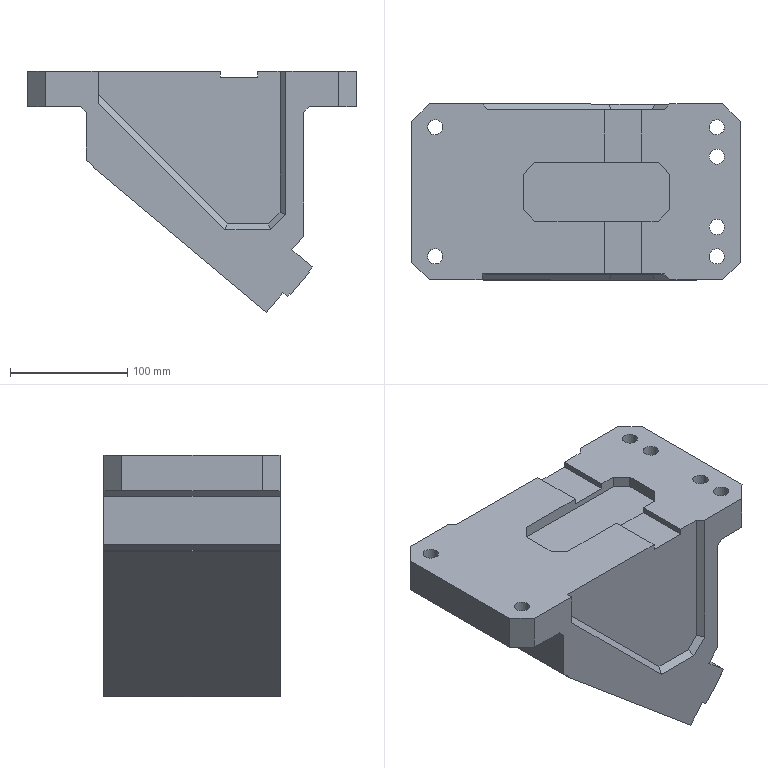Part | NX | features solid 2 | 1 solid | 69 faces | box 280 x 150 x 205.536 mm | volume 4318903 mm3 | plane 59 | cylinder 10 | commonest cylinder face diameters 13 x6 20 x4